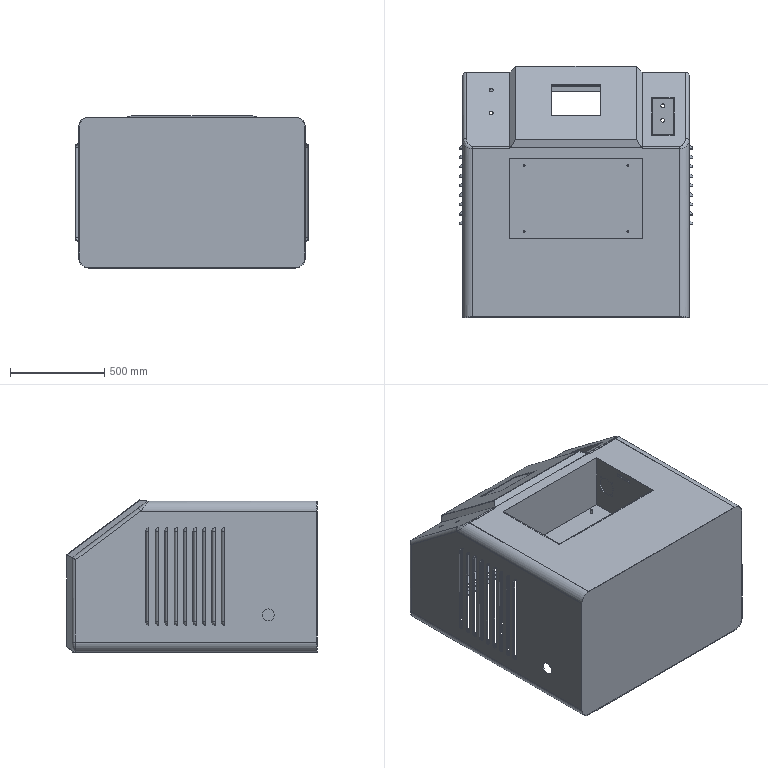Part | SolidWorks | features ICE 18, Cut 7, Fillet 4, Chamfer 2, MirrorPattern 2, Shell 2, Extrusion 1, LPattern 1 | 2 solids | 334 faces | box 1240 x 1330 x 806 mm | volume 19071542 mm3 | plane 132 | cylinder 104 | sphere 90 | torus 4 | spline 4 | commonest cylinder face diameters 40 x32 34 x26 10 x8 3.6 x6 7 x4 20 x4